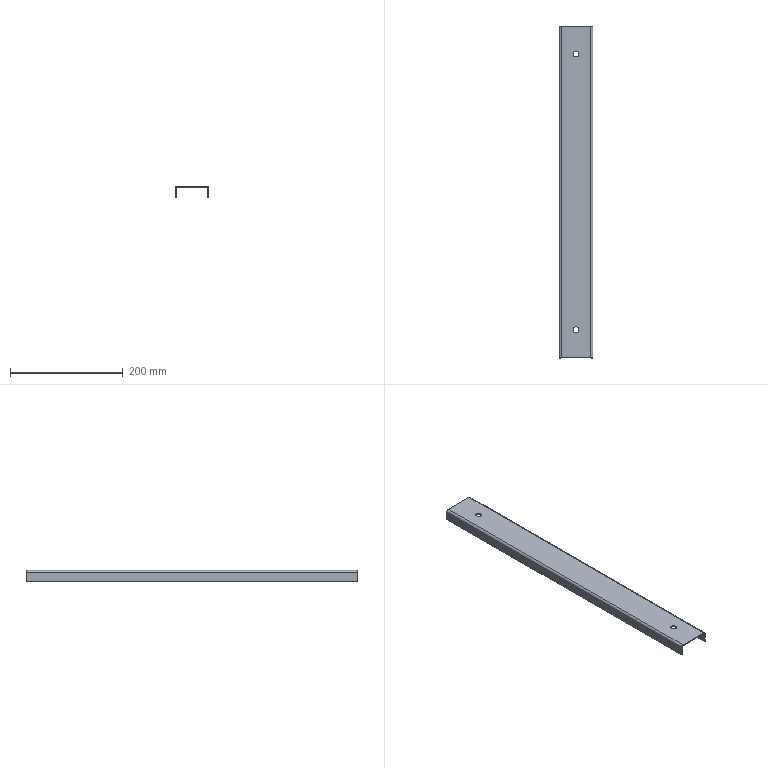Part | NX | features solid 2 | 1 solid | 18 faces | box 60 x 590 x 20 mm | volume 109914 mm3 | plane 10 | cylinder 8 | commonest cylinder face diameters 10.2 x4 4 x2 8 x2
STEP:
#1=CARTESIAN_POINT('',(-544.9,-570.,1293.));
#2=VERTEX_POINT('',#1);
#3=CARTESIAN_POINT('',(-544.9,-570.,1295.));
#4=VERTEX_POINT('',#3);
#5=CARTESIAN_POINT('',(-544.9,-570.,701.62));
#6=DIRECTION('',(0.,0.,1.));
#7=VECTOR('',#6,1000.);
#8=LINE('',#5,#7);
#9=EDGE_CURVE('',#2,#4,#8,.T.);
#10=ORIENTED_EDGE('',*,*,#9,.F.);
#11=CARTESIAN_POINT('',(-555.1,-570.,1293.));
#12=VERTEX_POINT('',#11);
#13=CARTESIAN_POINT('',(-550.,-570.,1293.));
#14=DIRECTION('',(0.,0.,-1.));
#15=DIRECTION('',(1.,0.,0.));
#16=AXIS2_PLACEMENT_3D('',#13,#14,#15);
#17=CIRCLE('',#16,5.1);
#18=EDGE_CURVE('',#2,#12,#17,.T.);
#19=ORIENTED_EDGE('',*,*,#18,.T.);
#20=CARTESIAN_POINT('',(-555.1,-570.,1295.));
#21=VERTEX_POINT('',#20);
#22=CARTESIAN_POINT('',(-555.1,-570.,701.62));
#23=DIRECTION('',(0.,0.,1.));
#24=VECTOR('',#23,1000.);
#25=LINE('',#22,#24);
#26=EDGE_CURVE('',#21,#12,#25,.F.);
#27=ORIENTED_EDGE('',*,*,#26,.F.);
#28=CARTESIAN_POINT('',(-550.,-570.,1295.));
#29=DIRECTION('',(0.,0.,1.));
#30=DIRECTION('',(0.,1.,0.));
#31=AXIS2_PLACEMENT_3D('',#28,#29,#30);
#32=CIRCLE('',#31,5.1);
#33=EDGE_CURVE('',#21,#4,#32,.T.);
#34=ORIENTED_EDGE('',*,*,#33,.T.);
#35=EDGE_LOOP('',(#10,#19,#27,#34));
#36=FACE_BOUND('',#35,.T.);
#37=CARTESIAN_POINT('',(-550.,-570.,701.62));
#38=DIRECTION('',(0.,0.,1.));
#39=DIRECTION('',(-1.,0.,0.));
#40=AXIS2_PLACEMENT_3D('',#37,#38,#39);
#41=CYLINDRICAL_SURFACE('',#40,5.1);
#42=ADVANCED_FACE('',(#36),#41,.F.);
#43=CARTESIAN_POINT('',(-544.9,-80.,1295.));
#44=VERTEX_POINT('',#43);
#45=CARTESIAN_POINT('',(-544.9,-80.,1293.));
#46=VERTEX_POINT('',#45);
#47=CARTESIAN_POINT('',(-544.9,-80.,701.62));
#48=DIRECTION('',(0.,0.,1.));
#49=VECTOR('',#48,1000.);
#50=LINE('',#47,#49);
#51=EDGE_CURVE('',#44,#46,#50,.F.);
#52=ORIENTED_EDGE('',*,*,#51,.T.);
#53=CARTESIAN_POINT('',(-555.1,-80.,1293.));
#54=VERTEX_POINT('',#53);
#55=CARTESIAN_POINT('',(-550.,-80.,1293.));
#56=DIRECTION('',(0.,0.,-1.));
#57=DIRECTION('',(1.,0.,0.));
#58=AXIS2_PLACEMENT_3D('',#55,#56,#57);
#59=CIRCLE('',#58,5.1);
#60=EDGE_CURVE('',#46,#54,#59,.T.);
#61=ORIENTED_EDGE('',*,*,#60,.T.);
#62=CARTESIAN_POINT('',(-555.1,-80.,1295.));
#63=VERTEX_POINT('',#62);
#64=CARTESIAN_POINT('',(-555.1,-80.,701.62));
#65=DIRECTION('',(0.,0.,1.));
#66=VECTOR('',#65,1000.);
#67=LINE('',#64,#66);
#68=EDGE_CURVE('',#54,#63,#67,.T.);
#69=ORIENTED_EDGE('',*,*,#68,.T.);
#70=CARTESIAN_POINT('',(-550.,-80.,1295.));
#71=DIRECTION('',(0.,0.,1.));
#72=DIRECTION('',(0.,1.,0.));
#73=AXIS2_PLACEMENT_3D('',#70,#71,#72);
#74=CIRCLE('',#73,5.1);
#75=EDGE_CURVE('',#63,#44,#74,.T.);
#76=ORIENTED_EDGE('',*,*,#75,.T.);
#77=EDGE_LOOP('',(#52,#61,#69,#76));
#78=FACE_BOUND('',#77,.T.);
#79=CARTESIAN_POINT('',(-550.,-80.,701.62));
#80=DIRECTION('',(0.,0.,1.));
#81=DIRECTION('',(-1.,0.,0.));
#82=AXIS2_PLACEMENT_3D('',#79,#80,#81);
#83=CYLINDRICAL_SURFACE('',#82,5.1);
#84=ADVANCED_FACE('',(#78),#83,.F.);
#85=CARTESIAN_POINT('',(-580.,-30.,1291.));
#86=VERTEX_POINT('',#85);
#87=CARTESIAN_POINT('',(-580.,-30.,1275.));
#88=VERTEX_POINT('',#87);
#89=CARTESIAN_POINT('',(-580.,-30.,1295.));
#90=DIRECTION('',(0.,0.,-1.));
#91=VECTOR('',#90,1000.);
#92=LINE('',#89,#91);
#93=EDGE_CURVE('',#86,#88,#92,.T.);
#94=ORIENTED_EDGE('',*,*,#93,.T.);
#95=CARTESIAN_POINT('',(-580.,-620.,1275.));
#96=VERTEX_POINT('',#95);
#97=CARTESIAN_POINT('',(-580.,-620.,1275.));
#98=DIRECTION('',(0.,1.,0.));
#99=VECTOR('',#98,1000.);
#100=LINE('',#97,#99);
#101=EDGE_CURVE('',#96,#88,#100,.T.);
#102=ORIENTED_EDGE('',*,*,#101,.F.);
#103=CARTESIAN_POINT('',(-580.,-620.,1291.));
#104=VERTEX_POINT('',#103);
#105=CARTESIAN_POINT('',(-580.,-620.,1295.));
#106=DIRECTION('',(0.,0.,-1.));
#107=VECTOR('',#106,1000.);
#108=LINE('',#105,#107);
#109=EDGE_CURVE('',#104,#96,#108,.T.);
#110=ORIENTED_EDGE('',*,*,#109,.F.);
#111=CARTESIAN_POINT('',(-580.,-620.,1291.));
#112=DIRECTION('',(0.,1.,0.));
#113=VECTOR('',#112,1000.);
#114=LINE('',#111,#113);
#115=EDGE_CURVE('',#104,#86,#114,.T.);
#116=ORIENTED_EDGE('',*,*,#115,.T.);
#117=EDGE_LOOP('',(#94,#102,#110,#116));
#118=FACE_BOUND('',#117,.T.);
#119=CARTESIAN_POINT('',(-580.,-620.,1295.));
#120=DIRECTION('',(1.,0.,0.));
#121=DIRECTION('',(0.,1.,0.));
#122=AXIS2_PLACEMENT_3D('',#119,#120,#121);
#123=PLANE('',#122);
#124=ADVANCED_FACE('',(#118),#123,.F.);
#125=CARTESIAN_POINT('',(-576.,-30.,1295.));
#126=VERTEX_POINT('',#125);
#127=CARTESIAN_POINT('',(-576.,-30.,1291.));
#128=DIRECTION('',(0.,-1.,0.));
#129=DIRECTION('',(0.,0.,-1.));
#130=AXIS2_PLACEMENT_3D('',#127,#128,#129);
#131=CIRCLE('',#130,4.);
#132=EDGE_CURVE('',#126,#86,#131,.T.);
#133=ORIENTED_EDGE('',*,*,#132,.T.);
#134=ORIENTED_EDGE('',*,*,#115,.F.);
#135=CARTESIAN_POINT('',(-576.,-620.,1295.));
#136=VERTEX_POINT('',#135);
#137=CARTESIAN_POINT('',(-576.,-620.,1291.));
#138=DIRECTION('',(0.,-1.,0.));
#139=DIRECTION('',(0.,0.,-1.));
#140=AXIS2_PLACEMENT_3D('',#137,#138,#139);
#141=CIRCLE('',#140,4.);
#142=EDGE_CURVE('',#136,#104,#141,.T.);
#143=ORIENTED_EDGE('',*,*,#142,.F.);
#144=CARTESIAN_POINT('',(-576.,-620.,1295.));
#145=DIRECTION('',(0.,1.,0.));
#146=VECTOR('',#145,1000.);
#147=LINE('',#144,#146);
#148=EDGE_CURVE('',#136,#126,#147,.T.);
#149=ORIENTED_EDGE('',*,*,#148,.T.);
#150=EDGE_LOOP('',(#133,#134,#143,#149));
#151=FACE_BOUND('',#150,.T.);
#152=CARTESIAN_POINT('',(-576.,-620.,1291.));
#153=DIRECTION('',(0.,1.,0.));
#154=DIRECTION('',(0.,0.,-1.));
#155=AXIS2_PLACEMENT_3D('',#152,#153,#154);
#156=CYLINDRICAL_SURFACE('',#155,4.);
#157=ADVANCED_FACE('',(#151),#156,.T.);
#158=ORIENTED_EDGE('',*,*,#75,.F.);
#159=CARTESIAN_POINT('',(-550.,-80.,1295.));
#160=DIRECTION('',(0.,0.,1.));
#161=DIRECTION('',(0.,1.,0.));
#162=AXIS2_PLACEMENT_3D('',#159,#160,#161);
#163=CIRCLE('',#162,5.1);
#164=EDGE_CURVE('',#44,#63,#163,.T.);
#165=ORIENTED_EDGE('',*,*,#164,.F.);
#166=EDGE_LOOP('',(#158,#165));
#167=FACE_BOUND('',#166,.T.);
#168=ORIENTED_EDGE('',*,*,#33,.F.);
#169=CARTESIAN_POINT('',(-550.,-570.,1295.));
#170=DIRECTION('',(0.,0.,1.));
#171=DIRECTION('',(0.,1.,0.));
#172=AXIS2_PLACEMENT_3D('',#169,#170,#171);
#173=CIRCLE('',#172,5.1);
#174=EDGE_CURVE('',#4,#21,#173,.T.);
#175=ORIENTED_EDGE('',*,*,#174,.F.);
#176=EDGE_LOOP('',(#168,#175));
#177=FACE_BOUND('',#176,.T.);
#178=CARTESIAN_POINT('',(-524.,-30.,1295.));
#179=VERTEX_POINT('',#178);
#180=CARTESIAN_POINT('',(-520.,-30.,1295.));
#181=DIRECTION('',(-1.,0.,0.));
#182=VECTOR('',#181,1000.);
#183=LINE('',#180,#182);
#184=EDGE_CURVE('',#179,#126,#183,.T.);
#185=ORIENTED_EDGE('',*,*,#184,.T.);
#186=ORIENTED_EDGE('',*,*,#148,.F.);
#187=CARTESIAN_POINT('',(-524.,-620.,1295.));
#188=VERTEX_POINT('',#187);
#189=CARTESIAN_POINT('',(-520.,-620.,1295.));
#190=DIRECTION('',(-1.,0.,0.));
#191=VECTOR('',#190,1000.);
#192=LINE('',#189,#191);
#193=EDGE_CURVE('',#188,#136,#192,.T.);
#194=ORIENTED_EDGE('',*,*,#193,.F.);
#195=CARTESIAN_POINT('',(-524.,-620.,1295.));
#196=DIRECTION('',(0.,1.,0.));
#197=VECTOR('',#196,1000.);
#198=LINE('',#195,#197);
#199=EDGE_CURVE('',#188,#179,#198,.T.);
#200=ORIENTED_EDGE('',*,*,#199,.T.);
#201=EDGE_LOOP('',(#185,#186,#194,#200));
#202=FACE_BOUND('',#201,.T.);
#203=CARTESIAN_POINT('',(-520.,-620.,1295.));
#204=DIRECTION('',(0.,0.,-1.));
#205=DIRECTION('',(-1.,0.,0.));
#206=AXIS2_PLACEMENT_3D('',#203,#204,#205);
#207=PLANE('',#206);
#208=ADVANCED_FACE('',(#167,#177,#202),#207,.F.);
#209=CARTESIAN_POINT('',(-520.,-30.,1291.));
#210=VERTEX_POINT('',#209);
#211=CARTESIAN_POINT('',(-524.,-30.,1291.));
#212=DIRECTION('',(0.,-1.,0.));
#213=DIRECTION('',(0.,0.,-1.));
#214=AXIS2_PLACEMENT_3D('',#211,#212,#213);
#215=CIRCLE('',#214,4.);
#216=EDGE_CURVE('',#210,#179,#215,.T.);
#217=ORIENTED_EDGE('',*,*,#216,.T.);
#218=ORIENTED_EDGE('',*,*,#199,.F.);
#219=CARTESIAN_POINT('',(-520.,-620.,1291.));
#220=VERTEX_POINT('',#219);
#221=CARTESIAN_POINT('',(-524.,-620.,1291.));
#222=DIRECTION('',(0.,-1.,0.));
#223=DIRECTION('',(0.,0.,-1.));
#224=AXIS2_PLACEMENT_3D('',#221,#222,#223);
#225=CIRCLE('',#224,4.);
#226=EDGE_CURVE('',#220,#188,#225,.T.);
#227=ORIENTED_EDGE('',*,*,#226,.F.);
#228=CARTESIAN_POINT('',(-520.,-620.,1291.));
#229=DIRECTION('',(0.,1.,0.));
#230=VECTOR('',#229,1000.);
#231=LINE('',#228,#230);
#232=EDGE_CURVE('',#220,#210,#231,.T.);
#233=ORIENTED_EDGE('',*,*,#232,.T.);
#234=EDGE_LOOP('',(#217,#218,#227,#233));
#235=FACE_BOUND('',#234,.T.);
#236=CARTESIAN_POINT('',(-524.,-620.,1291.));
#237=DIRECTION('',(0.,1.,0.));
#238=DIRECTION('',(0.,0.,-1.));
#239=AXIS2_PLACEMENT_3D('',#236,#237,#238);
#240=CYLINDRICAL_SURFACE('',#239,4.);
#241=ADVANCED_FACE('',(#235),#240,.T.);
#242=CARTESIAN_POINT('',(-520.,-30.,1275.));
#243=VERTEX_POINT('',#242);
#244=CARTESIAN_POINT('',(-520.,-30.,1275.));
#245=DIRECTION('',(0.,0.,1.));
#246=VECTOR('',#245,1000.);
#247=LINE('',#244,#246);
#248=EDGE_CURVE('',#243,#210,#247,.T.);
#249=ORIENTED_EDGE('',*,*,#248,.T.);
#250=ORIENTED_EDGE('',*,*,#232,.F.);
#251=CARTESIAN_POINT('',(-520.,-620.,1275.));
#252=VERTEX_POINT('',#251);
#253=CARTESIAN_POINT('',(-520.,-620.,1275.));
#254=DIRECTION('',(0.,0.,1.));
#255=VECTOR('',#254,1000.);
#256=LINE('',#253,#255);
#257=EDGE_CURVE('',#252,#220,#256,.T.);
#258=ORIENTED_EDGE('',*,*,#257,.F.);
#259=CARTESIAN_POINT('',(-520.,-620.,1275.));
#260=DIRECTION('',(0.,1.,0.));
#261=VECTOR('',#260,1000.);
#262=LINE('',#259,#261);
#263=EDGE_CURVE('',#252,#243,#262,.T.);
#264=ORIENTED_EDGE('',*,*,#263,.T.);
#265=EDGE_LOOP('',(#249,#250,#258,#264));
#266=FACE_BOUND('',#265,.T.);
#267=CARTESIAN_POINT('',(-520.,-620.,1275.));
#268=DIRECTION('',(-1.,0.,0.));
#269=DIRECTION('',(0.,1.,0.));
#270=AXIS2_PLACEMENT_3D('',#267,#268,#269);
#271=PLANE('',#270);
#272=ADVANCED_FACE('',(#266),#271,.F.);
#273=CARTESIAN_POINT('',(-578.,-30.,1291.));
#274=VERTEX_POINT('',#273);
#275=CARTESIAN_POINT('',(-578.,-30.,1275.));
#276=VERTEX_POINT('',#275);
#277=CARTESIAN_POINT('',(-578.,-30.,1295.));
#278=DIRECTION('',(0.,0.,-1.));
#279=VECTOR('',#278,1000.);
#280=LINE('',#277,#279);
#281=EDGE_CURVE('',#274,#276,#280,.T.);
#282=ORIENTED_EDGE('',*,*,#281,.F.);
#283=CARTESIAN_POINT('',(-578.,-620.,1291.));
#284=VERTEX_POINT('',#283);
#285=CARTESIAN_POINT('',(-578.,-620.,1291.));
#286=DIRECTION('',(0.,1.,0.));
#287=VECTOR('',#286,1000.);
#288=LINE('',#285,#287);
#289=EDGE_CURVE('',#284,#274,#288,.T.);
#290=ORIENTED_EDGE('',*,*,#289,.F.);
#291=CARTESIAN_POINT('',(-578.,-620.,1275.));
#292=VERTEX_POINT('',#291);
#293=CARTESIAN_POINT('',(-578.,-620.,1295.));
#294=DIRECTION('',(0.,0.,-1.));
#295=VECTOR('',#294,1000.);
#296=LINE('',#293,#295);
#297=EDGE_CURVE('',#284,#292,#296,.T.);
#298=ORIENTED_EDGE('',*,*,#297,.T.);
#299=CARTESIAN_POINT('',(-578.,-620.,1275.));
#300=DIRECTION('',(0.,1.,0.));
#301=VECTOR('',#300,1000.);
#302=LINE('',#299,#301);
#303=EDGE_CURVE('',#292,#276,#302,.T.);
#304=ORIENTED_EDGE('',*,*,#303,.T.);
#305=EDGE_LOOP('',(#282,#290,#298,#304));
#306=FACE_BOUND('',#305,.T.);
#307=CARTESIAN_POINT('',(-578.,-620.,1295.));
#308=DIRECTION('',(1.,0.,0.));
#309=DIRECTION('',(0.,1.,0.));
#310=AXIS2_PLACEMENT_3D('',#307,#308,#309);
#311=PLANE('',#310);
#312=ADVANCED_FACE('',(#306),#311,.T.);
#313=CARTESIAN_POINT('',(-576.,-30.,1293.));
#314=VERTEX_POINT('',#313);
#315=CARTESIAN_POINT('',(-576.,-30.,1291.));
#316=DIRECTION('',(0.,-1.,0.));
#317=DIRECTION('',(0.,0.,-1.));
#318=AXIS2_PLACEMENT_3D('',#315,#316,#317);
#319=CIRCLE('',#318,2.);
#320=EDGE_CURVE('',#314,#274,#319,.T.);
#321=ORIENTED_EDGE('',*,*,#320,.F.);
#322=CARTESIAN_POINT('',(-576.,-620.,1293.));
#323=VERTEX_POINT('',#322);
#324=CARTESIAN_POINT('',(-576.,-620.,1293.));
#325=DIRECTION('',(0.,1.,0.));
#326=VECTOR('',#325,1000.);
#327=LINE('',#324,#326);
#328=EDGE_CURVE('',#323,#314,#327,.T.);
#329=ORIENTED_EDGE('',*,*,#328,.F.);
#330=CARTESIAN_POINT('',(-576.,-620.,1291.));
#331=DIRECTION('',(0.,-1.,0.));
#332=DIRECTION('',(0.,0.,-1.));
#333=AXIS2_PLACEMENT_3D('',#330,#331,#332);
#334=CIRCLE('',#333,2.);
#335=EDGE_CURVE('',#323,#284,#334,.T.);
#336=ORIENTED_EDGE('',*,*,#335,.T.);
#337=ORIENTED_EDGE('',*,*,#289,.T.);
#338=EDGE_LOOP('',(#321,#329,#336,#337));
#339=FACE_BOUND('',#338,.T.);
#340=CARTESIAN_POINT('',(-576.,-620.,1291.));
#341=DIRECTION('',(0.,1.,0.));
#342=DIRECTION('',(0.,0.,-1.));
#343=AXIS2_PLACEMENT_3D('',#340,#341,#342);
#344=CYLINDRICAL_SURFACE('',#343,2.);
#345=ADVANCED_FACE('',(#339),#344,.F.);
#346=CARTESIAN_POINT('',(-550.,-80.,1293.));
#347=DIRECTION('',(0.,0.,-1.));
#348=DIRECTION('',(1.,0.,0.));
#349=AXIS2_PLACEMENT_3D('',#346,#347,#348);
#350=CIRCLE('',#349,5.1);
#351=EDGE_CURVE('',#54,#46,#350,.T.);
#352=ORIENTED_EDGE('',*,*,#351,.F.);
#353=ORIENTED_EDGE('',*,*,#60,.F.);
#354=EDGE_LOOP('',(#352,#353));
#355=FACE_BOUND('',#354,.T.);
#356=CARTESIAN_POINT('',(-550.,-570.,1293.));
#357=DIRECTION('',(0.,0.,-1.));
#358=DIRECTION('',(1.,0.,0.));
#359=AXIS2_PLACEMENT_3D('',#356,#357,#358);
#360=CIRCLE('',#359,5.1);
#361=EDGE_CURVE('',#12,#2,#360,.T.);
#362=ORIENTED_EDGE('',*,*,#361,.F.);
#363=ORIENTED_EDGE('',*,*,#18,.F.);
#364=EDGE_LOOP('',(#362,#363));
#365=FACE_BOUND('',#364,.T.);
#366=CARTESIAN_POINT('',(-524.,-30.,1293.));
#367=VERTEX_POINT('',#366);
#368=CARTESIAN_POINT('',(-520.,-30.,1293.));
#369=DIRECTION('',(-1.,0.,0.));
#370=VECTOR('',#369,1000.);
#371=LINE('',#368,#370);
#372=EDGE_CURVE('',#367,#314,#371,.T.);
#373=ORIENTED_EDGE('',*,*,#372,.F.);
#374=CARTESIAN_POINT('',(-524.,-620.,1293.));
#375=VERTEX_POINT('',#374);
#376=CARTESIAN_POINT('',(-524.,-620.,1293.));
#377=DIRECTION('',(0.,1.,0.));
#378=VECTOR('',#377,1000.);
#379=LINE('',#376,#378);
#380=EDGE_CURVE('',#375,#367,#379,.T.);
#381=ORIENTED_EDGE('',*,*,#380,.F.);
#382=CARTESIAN_POINT('',(-520.,-620.,1293.));
#383=DIRECTION('',(-1.,0.,0.));
#384=VECTOR('',#383,1000.);
#385=LINE('',#382,#384);
#386=EDGE_CURVE('',#375,#323,#385,.T.);
#387=ORIENTED_EDGE('',*,*,#386,.T.);
#388=ORIENTED_EDGE('',*,*,#328,.T.);
#389=EDGE_LOOP('',(#373,#381,#387,#388));
#390=FACE_BOUND('',#389,.T.);
#391=CARTESIAN_POINT('',(-520.,-620.,1293.));
#392=DIRECTION('',(0.,0.,-1.));
#393=DIRECTION('',(-1.,0.,0.));
#394=AXIS2_PLACEMENT_3D('',#391,#392,#393);
#395=PLANE('',#394);
#396=ADVANCED_FACE('',(#355,#365,#390),#395,.T.);
#397=CARTESIAN_POINT('',(-522.,-30.,1291.));
#398=VERTEX_POINT('',#397);
#399=CARTESIAN_POINT('',(-524.,-30.,1291.));
#400=DIRECTION('',(0.,-1.,0.));
#401=DIRECTION('',(0.,0.,-1.));
#402=AXIS2_PLACEMENT_3D('',#399,#400,#401);
#403=CIRCLE('',#402,2.);
#404=EDGE_CURVE('',#398,#367,#403,.T.);
#405=ORIENTED_EDGE('',*,*,#404,.F.);
#406=CARTESIAN_POINT('',(-522.,-620.,1291.));
#407=VERTEX_POINT('',#406);
#408=CARTESIAN_POINT('',(-522.,-620.,1291.));
#409=DIRECTION('',(0.,1.,0.));
#410=VECTOR('',#409,1000.);
#411=LINE('',#408,#410);
#412=EDGE_CURVE('',#407,#398,#411,.T.);
#413=ORIENTED_EDGE('',*,*,#412,.F.);
#414=CARTESIAN_POINT('',(-524.,-620.,1291.));
#415=DIRECTION('',(0.,-1.,0.));
#416=DIRECTION('',(0.,0.,-1.));
#417=AXIS2_PLACEMENT_3D('',#414,#415,#416);
#418=CIRCLE('',#417,2.);
#419=EDGE_CURVE('',#407,#375,#418,.T.);
#420=ORIENTED_EDGE('',*,*,#419,.T.);
#421=ORIENTED_EDGE('',*,*,#380,.T.);
#422=EDGE_LOOP('',(#405,#413,#420,#421));
#423=FACE_BOUND('',#422,.T.);
#424=CARTESIAN_POINT('',(-524.,-620.,1291.));
#425=DIRECTION('',(0.,1.,0.));
#426=DIRECTION('',(0.,0.,-1.));
#427=AXIS2_PLACEMENT_3D('',#424,#425,#426);
#428=CYLINDRICAL_SURFACE('',#427,2.);
#429=ADVANCED_FACE('',(#423),#428,.F.);
#430=CARTESIAN_POINT('',(-522.,-30.,1275.));
#431=VERTEX_POINT('',#430);
#432=CARTESIAN_POINT('',(-522.,-30.,1275.));
#433=DIRECTION('',(0.,0.,1.));
#434=VECTOR('',#433,1000.);
#435=LINE('',#432,#434);
#436=EDGE_CURVE('',#431,#398,#435,.T.);
#437=ORIENTED_EDGE('',*,*,#436,.F.);
#438=CARTESIAN_POINT('',(-522.,-620.,1275.));
#439=VERTEX_POINT('',#438);
#440=CARTESIAN_POINT('',(-522.,-620.,1275.));
#441=DIRECTION('',(0.,1.,0.));
#442=VECTOR('',#441,1000.);
#443=LINE('',#440,#442);
#444=EDGE_CURVE('',#439,#431,#443,.T.);
#445=ORIENTED_EDGE('',*,*,#444,.F.);
#446=CARTESIAN_POINT('',(-522.,-620.,1275.));
#447=DIRECTION('',(0.,0.,1.));
#448=VECTOR('',#447,1000.);
#449=LINE('',#446,#448);
#450=EDGE_CURVE('',#439,#407,#449,.T.);
#451=ORIENTED_EDGE('',*,*,#450,.T.);
#452=ORIENTED_EDGE('',*,*,#412,.T.);
#453=EDGE_LOOP('',(#437,#445,#451,#452));
#454=FACE_BOUND('',#453,.T.);
#455=CARTESIAN_POINT('',(-522.,-620.,1275.));
#456=DIRECTION('',(-1.,0.,0.));
#457=DIRECTION('',(0.,1.,0.));
#458=AXIS2_PLACEMENT_3D('',#455,#456,#457);
#459=PLANE('',#458);
#460=ADVANCED_FACE('',(#454),#459,.T.);
#461=ORIENTED_EDGE('',*,*,#263,.F.);
#462=CARTESIAN_POINT('',(-520.,-620.,1275.));
#463=DIRECTION('',(-1.,0.,0.));
#464=VECTOR('',#463,1000.);
#465=LINE('',#462,#464);
#466=EDGE_CURVE('',#252,#439,#465,.T.);
#467=ORIENTED_EDGE('',*,*,#466,.T.);
#468=ORIENTED_EDGE('',*,*,#444,.T.);
#469=CARTESIAN_POINT('',(-520.,-30.,1275.));
#470=DIRECTION('',(-1.,0.,0.));
#471=VECTOR('',#470,1000.);
#472=LINE('',#469,#471);
#473=EDGE_CURVE('',#243,#431,#472,.T.);
#474=ORIENTED_EDGE('',*,*,#473,.F.);
#475=EDGE_LOOP('',(#461,#467,#468,#474));
#476=FACE_BOUND('',#475,.T.);
#477=CARTESIAN_POINT('',(-520.,-620.,1275.));
#478=DIRECTION('',(0.,0.,1.));
#479=DIRECTION('',(1.,0.,0.));
#480=AXIS2_PLACEMENT_3D('',#477,#478,#479);
#481=PLANE('',#480);
#482=ADVANCED_FACE('',(#476),#481,.F.);
#483=ORIENTED_EDGE('',*,*,#436,.T.);
#484=ORIENTED_EDGE('',*,*,#404,.T.);
#485=ORIENTED_EDGE('',*,*,#372,.T.);
#486=ORIENTED_EDGE('',*,*,#320,.T.);
#487=ORIENTED_EDGE('',*,*,#281,.T.);
#488=CARTESIAN_POINT('',(-580.,-30.,1275.));
#489=DIRECTION('',(1.,0.,0.));
#490=VECTOR('',#489,1000.);
#491=LINE('',#488,#490);
#492=EDGE_CURVE('',#88,#276,#491,.T.);
#493=ORIENTED_EDGE('',*,*,#492,.F.);
#494=ORIENTED_EDGE('',*,*,#93,.F.);
#495=ORIENTED_EDGE('',*,*,#132,.F.);
#496=ORIENTED_EDGE('',*,*,#184,.F.);
#497=ORIENTED_EDGE('',*,*,#216,.F.);
#498=ORIENTED_EDGE('',*,*,#248,.F.);
#499=ORIENTED_EDGE('',*,*,#473,.T.);
#500=EDGE_LOOP('',(#483,#484,#485,#486,#487,#493,#494,#495,#496,#497,#498,#499));
#501=FACE_BOUND('',#500,.T.);
#502=CARTESIAN_POINT('',(-520.,-30.,1275.));
#503=DIRECTION('',(0.,-1.,0.));
#504=DIRECTION('',(0.,0.,-1.));
#505=AXIS2_PLACEMENT_3D('',#502,#503,#504);
#506=PLANE('',#505);
#507=ADVANCED_FACE('',(#501),#506,.F.);
#508=CARTESIAN_POINT('',(-580.,-620.,1275.));
#509=DIRECTION('',(1.,0.,0.));
#510=VECTOR('',#509,1000.);
#511=LINE('',#508,#510);
#512=EDGE_CURVE('',#96,#292,#511,.T.);
#513=ORIENTED_EDGE('',*,*,#512,.F.);
#514=ORIENTED_EDGE('',*,*,#101,.T.);
#515=ORIENTED_EDGE('',*,*,#492,.T.);
#516=ORIENTED_EDGE('',*,*,#303,.F.);
#517=EDGE_LOOP('',(#513,#514,#515,#516));
#518=FACE_BOUND('',#517,.T.);
#519=CARTESIAN_POINT('',(-580.,-620.,1275.));
#520=DIRECTION('',(0.,0.,-1.));
#521=DIRECTION('',(-1.,0.,0.));
#522=AXIS2_PLACEMENT_3D('',#519,#520,#521);
#523=PLANE('',#522);
#524=ADVANCED_FACE('',(#518),#523,.T.);
#525=ORIENTED_EDGE('',*,*,#297,.F.);
#526=ORIENTED_EDGE('',*,*,#335,.F.);
#527=ORIENTED_EDGE('',*,*,#386,.F.);
#528=ORIENTED_EDGE('',*,*,#419,.F.);
#529=ORIENTED_EDGE('',*,*,#450,.F.);
#530=ORIENTED_EDGE('',*,*,#466,.F.);
#531=ORIENTED_EDGE('',*,*,#257,.T.);
#532=ORIENTED_EDGE('',*,*,#226,.T.);
#533=ORIENTED_EDGE('',*,*,#193,.T.);
#534=ORIENTED_EDGE('',*,*,#142,.T.);
#535=ORIENTED_EDGE('',*,*,#109,.T.);
#536=ORIENTED_EDGE('',*,*,#512,.T.);
#537=EDGE_LOOP('',(#525,#526,#527,#528,#529,#530,#531,#532,#533,#534,#535,#536));
#538=FACE_BOUND('',#537,.T.);
#539=CARTESIAN_POINT('',(-580.,-620.,1295.));
#540=DIRECTION('',(0.,-1.,0.));
#541=DIRECTION('',(0.,0.,-1.));
#542=AXIS2_PLACEMENT_3D('',#539,#540,#541);
#543=PLANE('',#542);
#544=ADVANCED_FACE('',(#538),#543,.T.);
#545=ORIENTED_EDGE('',*,*,#351,.T.);
#546=ORIENTED_EDGE('',*,*,#51,.F.);
#547=ORIENTED_EDGE('',*,*,#164,.T.);
#548=ORIENTED_EDGE('',*,*,#68,.F.);
#549=EDGE_LOOP('',(#545,#546,#547,#548));
#550=FACE_BOUND('',#549,.T.);
#551=CARTESIAN_POINT('',(-550.,-80.,701.62));
#552=DIRECTION('',(0.,0.,1.));
#553=DIRECTION('',(-1.,0.,0.));
#554=AXIS2_PLACEMENT_3D('',#551,#552,#553);
#555=CYLINDRICAL_SURFACE('',#554,5.1);
#556=ADVANCED_FACE('',(#550),#555,.F.);
#557=ORIENTED_EDGE('',*,*,#361,.T.);
#558=ORIENTED_EDGE('',*,*,#9,.T.);
#559=ORIENTED_EDGE('',*,*,#174,.T.);
#560=ORIENTED_EDGE('',*,*,#26,.T.);
#561=EDGE_LOOP('',(#557,#558,#559,#560));
#562=FACE_BOUND('',#561,.T.);
#563=CARTESIAN_POINT('',(-550.,-570.,701.62));
#564=DIRECTION('',(0.,0.,1.));
#565=DIRECTION('',(-1.,0.,0.));
#566=AXIS2_PLACEMENT_3D('',#563,#564,#565);
#567=CYLINDRICAL_SURFACE('',#566,5.1);
#568=ADVANCED_FACE('',(#562),#567,.F.);
#569=CLOSED_SHELL('',(#42,#84,#124,#157,#208,#241,#272,#312,#345,#396,#429,#460,#482,#507,#524,#544,#556,#568));
#570=MANIFOLD_SOLID_BREP('',#569);
#571=(LENGTH_UNIT()NAMED_UNIT(*)SI_UNIT(.MILLI.,.METRE.));
#572=UNCERTAINTY_MEASURE_WITH_UNIT(LENGTH_MEASURE(0.00001),#571,'','');
#573=(NAMED_UNIT(*)PLANE_ANGLE_UNIT()SI_UNIT($,.RADIAN.));
#574=(NAMED_UNIT(*)SI_UNIT($,.STERADIAN.)SOLID_ANGLE_UNIT());
#575=(GEOMETRIC_REPRESENTATION_CONTEXT(3)GLOBAL_UNCERTAINTY_ASSIGNED_CONTEXT((#572))GLOBAL_UNIT_ASSIGNED_CONTEXT((#571,#573,#574))REPRESENTATION_CONTEXT('',''));
#576=ADVANCED_BREP_SHAPE_REPRESENTATION('',(#570),#575);